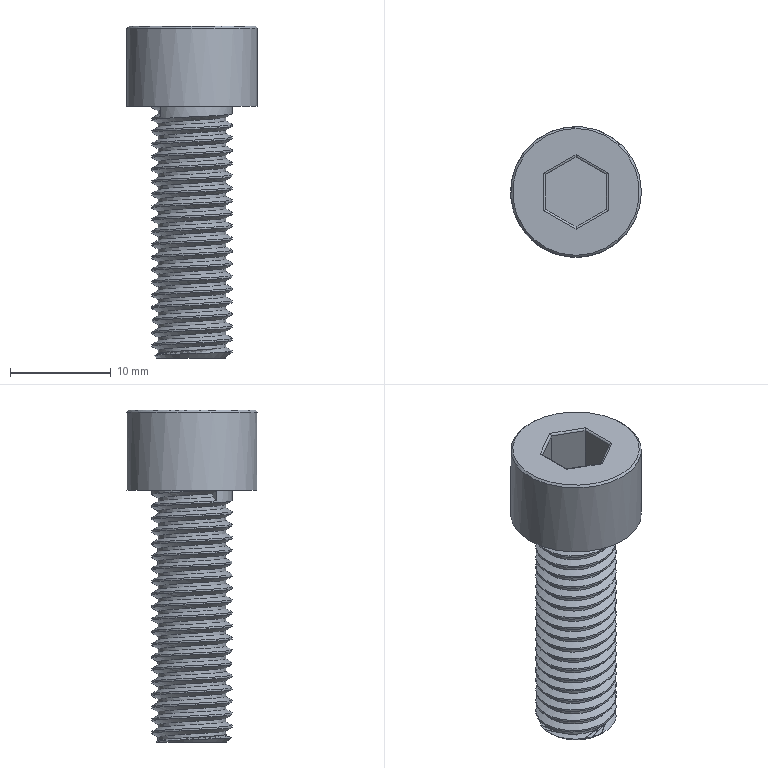Part | STEP file | Tube feed_id1742_x_t | 1 solid | 25 faces | box 13 x 13 x 33 mm | volume 1945 mm3 | plane 11 | cylinder 9 | spline 3 | torus 1 | cone 1 | commonest cylinder face diameters 0.4 x6 6.75 x1 8 x1 13 x1